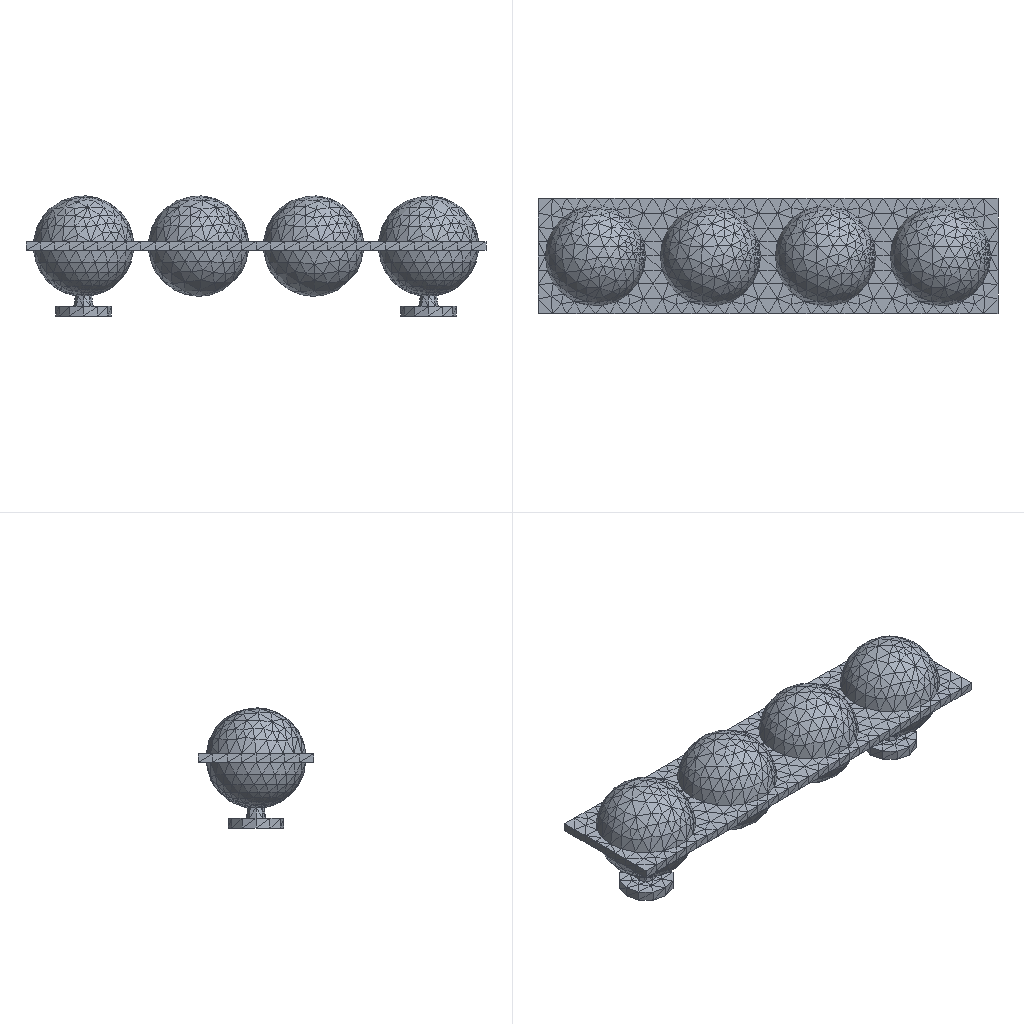Simulation study | abaqus
Set-up summary:
category,name,step,type,value,unit,region
solver,abaqus
solver,version,,,Abaqus/Standard 2020
units,not stated in the deck,,not stated
analysis,deck,,transient,transient
load_step,Step-1,Step-1,transient
load_step,Step-2,Step-2,transient
load_step,Step-3,Step-3,transient
load_step,Step-4,Step-4,transient
load_step,Step-5,Step-5,transient
load_step,Step-6,Step-6,transient
load_step,Step-7,Step-7,transient
load_step,Step-8,Step-8,transient
load_step,requested,,,8
mesh,nodes,,,2127
mesh,elements,,,6350
element_type,C3D4H,,solid,6350
load,load commands in deck,,count,10
bc,support commands in deck,,count,2
material,MATERIAL-1,,in results
check,setup vs results,,match,"per instance, exact: element labels, types and connectivity; labels of the nodes the elements use; coordinates of those nodes at SINGLE_PRECISION in 1 of 1 instance(s)"
Abaqus input file, long lists of numbers shortened:
*Heading
** Job name: Job-2 Model name: Model-1-Copy
** Generated by: Abaqus/CAE 2020
*Preprint, echo=NO, model=NO, history=NO, contact=NO
**
** PARTS
**
*Part, name=Part-4
*Node
      1,   116.804,           0.,  -34.854
      2,   123.196,           0.,  -34.854
** (2125 more lines like these left out)
*Element, type=C3D4H
   1, 2079, 2080,   17,   27
   2,  169, 2081, 1075, 1018
** (6348 more lines like these left out)
*Nset, nset=Set-4, generate
    1,  2127,     1
*Elset, elset=Set-4, generate
    1,  6350,     1
** Section: Section-1
*Solid Section, elset=Set-4, material=Material-1
,
*End Part
**
**
** ASSEMBLY
**
*Assembly, name=Assembly
**
*Instance, name=Part-4-1, part=Part-4
*End Instance
**
*Nset, nset=Set-1, instance=Part-4-1
  63,  64,  65,  66, 519, 520, 521, 522, 523, 524, 525, 526, 527, 528, 529, 530
 531, 532, 533, 534
*Elset, elset=Set-1, instance=Part-4-1
 3357, 3370, 3373, 3374, 3381, 3384, 3395, 3401, 3404, 3412, 3414, 3423, 3424, 3425, 3428, 3432
 3440, 3445, 3450, 3451
*Nset, nset=Set-2, instance=Part-4-1
   7,   8,   9,  10,  99, 100, 101, 102, 103, 104, 105, 106, 107, 108, 109, 110
 111, 112, 113, 114
*Elset, elset=Set-2, instance=Part-4-1
 2982, 2992, 2993, 3009, 3025, 3029, 3032, 3041, 3056, 3057, 3066, 3069, 3079, 3084, 3093, 3102
 3117, 3125, 3131, 3157
*Nset, nset=Set-3, instance=Part-4-1
  63,  64,  65,  66, 519, 520, 521, 522, 523, 524, 525, 526, 527, 528, 529, 530
 531, 532, 533, 534
*Elset, elset=Set-3, instance=Part-4-1
 3357, 3370, 3373, 3374, 3381, 3384, 3395, 3401, 3404, 3412, 3414, 3423, 3424, 3425, 3428, 3432
 3440, 3445, 3450, 3451
*Nset, nset=Set-4, instance=Part-4-1
   7,   8,   9,  10,  99, 100, 101, 102, 103, 104, 105, 106, 107, 108, 109, 110
 111, 112, 113, 114
*Elset, elset=Set-4, instance=Part-4-1
 2982, 2992, 2993, 3009, 3025, 3029, 3032, 3041, 3056, 3057, 3066, 3069, 3079, 3084, 3093, 3102
 3117, 3125, 3131, 3157
*Nset, nset=Set-5, instance=Part-4-1
  63,  64,  65,  66, 519, 520, 521, 522, 523, 524, 525, 526, 527, 528, 529, 530
 531, 532, 533, 534
*Elset, elset=Set-5, instance=Part-4-1
 3357, 3370, 3373, 3374, 3381, 3384, 3395, 3401, 3404, 3412, 3414, 3423, 3424, 3425, 3428, 3432
 3440, 3445, 3450, 3451
*Nset, nset=Set-6, instance=Part-4-1
   7,   8,   9,  10,  99, 100, 101, 102, 103, 104, 105, 106, 107, 108, 109, 110
 111, 112, 113, 114
*Elset, elset=Set-6, instance=Part-4-1
 2982, 2992, 2993, 3009, 3025, 3029, 3032, 3041, 3056, 3057, 3066, 3069, 3079, 3084, 3093, 3102
 3117, 3125, 3131, 3157
*Elset, elset=_Surf-1_S3, internal, instance=Part-4-1
   38,   82,   83,   98,  101,  102,  103,  178,  233,  238,  269,  271,  272, 1477, 1518, 1523
 1548, 1561, 1564, 1630, 1633, 1669, 1682, 1708, 1709, 1766, 1768, 1770, 1784, 1787, 1799, 1802
** (22 more lines like these left out)
*Elset, elset=_Surf-1_S4, internal, instance=Part-4-1
   39,   41,  630, 1513, 1600, 1821, 1840, 1843, 1905, 3464, 5248, 5324, 5368, 5438, 5474, 5518
 5533, 5703, 5804, 5953, 5978
*Elset, elset=_Surf-1_S1, internal, instance=Part-4-1
  236,  276, 1549, 1631, 1634, 1700, 2060, 2424, 3561, 5379, 5427, 5439, 5487, 5599, 5615, 5645
 5658, 5682, 5917, 5991
*Elset, elset=_Surf-1_S2, internal, instance=Part-4-1
  828, 1581, 1800, 1901, 1921, 1998, 2020, 2058, 2784, 5366, 5468, 5511, 5515, 5526, 5538, 5585
 5602, 5663, 5671, 5719, 5744, 5947, 5980, 6014
*Surface, type=ELEMENT, name=Surf-1
_Surf-1_S3, S3
_Surf-1_S4, S4
_Surf-1_S2, S2
_Surf-1_S1, S1
*Elset, elset=_Surf-2_S4, internal, instance=Part-4-1
   55,   57,   66, 2162, 2179, 2191, 2194, 2238, 2249, 2394, 2414, 2586, 2627, 2734, 2843, 3613
 3855, 3928, 3953, 3965, 3977, 4341, 4403, 4483
*Elset, elset=_Surf-2_S2, internal, instance=Part-4-1
   67, 1976, 2148, 2149, 2306, 2392, 2616, 2723, 2750, 2950, 2980, 3040, 3042, 3095, 3105, 3203
 3615, 3616, 3621, 3624, 3790, 3799, 3823, 3827, 3836, 3843, 3860, 3882, 3892, 3893, 3907, 3911
** (1 more lines like these left out)
*Elset, elset=_Surf-2_S3, internal, instance=Part-4-1
  148,  158,  248,  251,  252,  253,  255,  259,  262,  264,  266,  267,  268,  701, 1087, 2150
 2201, 2310, 2395, 2405, 2409, 2434, 2457, 2461, 2466, 2467, 2469, 2474, 2477, 2480, 2487, 2488
** (29 more lines like these left out)
*Elset, elset=_Surf-2_S1, internal, instance=Part-4-1
  149,  188,  256, 2313, 2339, 2730, 2775, 3481, 3612, 3883, 4087
*Surface, type=ELEMENT, name=Surf-2
_Surf-2_S4, S4
_Surf-2_S2, S2
_Surf-2_S3, S3
_Surf-2_S1, S1
*Elset, elset=_Surf-3_S3, internal, instance=Part-4-1
   26,   48,  141,  142,  171,  172,  173,  196,  197,  240,  242,  244,  245,  803,  804,  946
  947,  978, 1020, 1024, 1045, 1072, 1076, 1078, 1080, 1086, 1094, 1101, 1119, 1134, 1137, 1139
** (22 more lines like these left out)
*Elset, elset=_Surf-3_S4, internal, instance=Part-4-1
  131,  205,  642,  873,  884,  896,  921,  924,  977, 1002, 1035, 1093, 1100, 1175, 1227, 1268
 1425, 4412, 4523, 4536, 4668, 4775, 4796, 4799, 4893, 5139, 5172, 5711, 5914
*Elset, elset=_Surf-3_S2, internal, instance=Part-4-1
  169,  241, 1029, 1254, 1327, 4774, 4810, 4889, 5092, 5825, 5873, 6028, 6055
*Elset, elset=_Surf-3_S1, internal, instance=Part-4-1
  198,  201,  857,  950,  952, 1042, 1168, 1267, 1418, 4520, 4574, 4813, 4891, 4969, 5012, 5089
 5816, 5862
*Surface, type=ELEMENT, name=Surf-3
_Surf-3_S3, S3
_Surf-3_S4, S4
_Surf-3_S2, S2
_Surf-3_S1, S1
*Elset, elset=_Surf-4_S3, internal, instance=Part-4-1
   61,  109,  117,  225,  229,  232,  305,  319,  321,  351,  359,  384,  412,  413,  423,  424
  427,  436,  437,  444,  449,  484,  486,  495,  503,  510,  516,  518,  520,  555,  556,  560
** (30 more lines like these left out)
*Elset, elset=_Surf-4_S4, internal, instance=Part-4-1
    2,   28,  224,  297,  346,  396,  451,  540,  542,  563,  571,  778,  793, 1792, 2125, 2305
 2459, 2646, 3160, 4894, 5064, 5102, 5751, 5838, 6214, 6346
*Elset, elset=_Surf-4_S1, internal, instance=Part-4-1
   10,   59,  122,  442,  652,  659,  783,  840, 1036, 2777, 2986, 3729, 4063, 4506, 4542, 4947
 5945,
*Elset, elset=_Surf-4_S2, internal, instance=Part-4-1
  231,  781,  994, 1125, 1514, 1865, 2039, 2766, 2817, 2957, 3072, 3606, 3723, 4623, 4741, 4762
 4817, 4819, 4897, 5008, 5046, 5443, 6135, 6156, 6316
*Surface, type=ELEMENT, name=Surf-4
_Surf-4_S3, S3
_Surf-4_S4, S4
_Surf-4_S2, S2
_Surf-4_S1, S1
*Elset, elset=_Surf-6_S2, internal, instance=Part-4-1
  275, 1467, 1472, 1476, 1482, 1487, 1494, 1498, 1501, 1512, 1521, 1551, 1558, 1563, 1565, 1572
 1573, 1578, 1584, 1589, 1594, 1596, 1598, 1607, 1614, 1617, 1619, 1624, 1641, 1644, 1650, 1654
** (5 more lines like these left out)
*Elset, elset=_Surf-6_S4, internal, instance=Part-4-1
 1480, 1503, 1541, 1554, 1579, 1583, 1586, 1591, 1597, 1602, 1615, 1626, 1628, 1639, 1640, 1655
 1676, 1678, 1686, 1695, 1731, 1744, 1745, 1778, 1783, 1793, 1794, 1811, 1817, 1879, 1882, 1902
** (2 more lines like these left out)
*Elset, elset=_Surf-6_S1, internal, instance=Part-4-1
 1485, 1488, 1496, 1497, 1502, 1507, 1517, 1528, 1535, 1555, 1566, 1570, 1592, 1601, 1603, 1606
 1608, 1632, 1647, 1649, 1668, 1673, 1674, 1689, 1693, 1702, 1710, 1714, 1725, 1740, 1743, 1754
** (3 more lines like these left out)
*Elset, elset=_Surf-6_S3, internal, instance=Part-4-1
 1486, 1505, 1567, 1694, 1805, 1810, 1812, 1886, 1970, 1983, 2031, 2061, 5649
*Surface, type=ELEMENT, name=Surf-6
_Surf-6_S2, S2
_Surf-6_S4, S4
_Surf-6_S1, S1
_Surf-6_S3, S3
*Elset, elset=_Surf-9_S2, internal, instance=Part-4-1
  801,  806,  810,  819,  827,  831,  836,  849,  861,  862,  870,  871,  885,  889,  890,  899
  900,  908,  913,  915,  916,  919,  936,  937,  938,  939,  943,  945,  961,  968,  970,  972
** (5 more lines like these left out)
*Elset, elset=_Surf-9_S1, internal, instance=Part-4-1
  805,  807,  813,  814,  818,  829,  830,  833,  837,  847,  853,  859,  864,  866,  875,  886
  897,  902,  905,  931,  941,  956,  958,  959,  974,  984,  989, 1000, 1017, 1034, 1039, 1063
** (3 more lines like these left out)
*Elset, elset=_Surf-9_S4, internal, instance=Part-4-1
  809,  821,  839,  851,  868,  879,  909,  914,  935,  949,  951,  955,  965,  981, 1026, 1031
 1065, 1074, 1098, 1109, 1121, 1126, 1142, 1146, 1152, 1164, 1177, 1180, 1224, 1234, 1253, 1257
** (2 more lines like these left out)
*Elset, elset=_Surf-9_S3, internal, instance=Part-4-1
  838,  841,  966, 1122, 1155, 1205, 1311, 1316, 1344, 1458, 2728, 3870, 4904, 5887, 6086, 6122
*Surface, type=ELEMENT, name=Surf-9
_Surf-9_S2, S2
_Surf-9_S1, S1
_Surf-9_S4, S4
_Surf-9_S3, S3
*Elset, elset=_Surf-10_S2, internal, instance=Part-4-1
   78,  204,  309,  312,  313,  318,  320,  330,  339,  340,  347,  354,  355,  357,  360,  365
  372,  374,  382,  389,  398,  400,  406,  410,  414,  416,  422,  430,  443,  445,  460,  472
** (6 more lines like these left out)
*Elset, elset=_Surf-10_S4, internal, instance=Part-4-1
  307,  310,  325,  349,  353,  358,  361,  379,  405,  419,  426,  450,  464,  505,  521,  531
  535,  602,  614,  641,  653,  657,  679,  696,  734,  763,  768,  811,  933, 1033, 1240, 1575
** (2 more lines like these left out)
*Elset, elset=_Surf-10_S1, internal, instance=Part-4-1
  308,  331,  336,  367,  385,  397,  418,  428,  440,  448,  461,  478,  479,  501,  513,  517
  532,  546,  566,  569,  585,  590,  603,  609,  624,  631,  637,  656,  677,  685,  694,  699
** (3 more lines like these left out)
*Elset, elset=_Surf-10_S3, internal, instance=Part-4-1
  329,  363,  364,  465,  474,  538,  686,  698,  907, 1337, 2126, 2135, 5563, 6035, 6327
*Surface, type=ELEMENT, name=Surf-10
_Surf-10_S2, S2
_Surf-10_S4, S4
_Surf-10_S1, S1
_Surf-10_S3, S3
*Elset, elset=_Surf-12_S2, internal, instance=Part-4-1
   63,  749, 2142, 2151, 2157, 2159, 2161, 2182, 2193, 2211, 2214, 2223, 2230, 2234, 2237, 2246
 2247, 2251, 2252, 2261, 2269, 2276, 2284, 2304, 2322, 2326, 2330, 2331, 2341, 2343, 2346, 2350
** (5 more lines like these left out)
*Elset, elset=_Surf-12_S3, internal, instance=Part-4-1
  182, 2156, 2290, 2319, 2352, 2358, 2360, 2425, 2541, 2642, 2762, 2874, 3073, 3794
*Elset, elset=_Surf-12_S4, internal, instance=Part-4-1
 2144, 2165, 2204, 2207, 2228, 2235, 2242, 2253, 2258, 2273, 2280, 2281, 2287, 2295, 2308, 2309
 2311, 2314, 2316, 2348, 2408, 2411, 2444, 2482, 2498, 2520, 2529, 2557, 2609, 2640, 2655, 2715
** (2 more lines like these left out)
*Elset, elset=_Surf-12_S1, internal, instance=Part-4-1
 2147, 2160, 2167, 2168, 2187, 2188, 2189, 2195, 2209, 2212, 2215, 2233, 2259, 2267, 2271, 2288
 2289, 2298, 2321, 2337, 2340, 2355, 2368, 2383, 2415, 2418, 2440, 2450, 2517, 2532, 2537, 2558
** (3 more lines like these left out)
*Surface, type=ELEMENT, name=Surf-12
_Surf-12_S2, S2
_Surf-12_S3, S3
_Surf-12_S4, S4
_Surf-12_S1, S1
*Elset, elset=_Surf-13_S2, internal, instance=Part-4-1
  275, 1467, 1472, 1476, 1482, 1487, 1494, 1498, 1501, 1512, 1521, 1551, 1558, 1563, 1565, 1572
 1573, 1578, 1584, 1589, 1594, 1596, 1598, 1607, 1614, 1617, 1619, 1624, 1641, 1644, 1650, 1654
** (5 more lines like these left out)
*Elset, elset=_Surf-13_S4, internal, instance=Part-4-1
 1480, 1503, 1541, 1554, 1579, 1583, 1586, 1591, 1597, 1602, 1615, 1626, 1628, 1639, 1640, 1655
 1676, 1678, 1686, 1695, 1731, 1744, 1745, 1778, 1783, 1793, 1794, 1811, 1817, 1879, 1882, 1902
** (2 more lines like these left out)
*Elset, elset=_Surf-13_S1, internal, instance=Part-4-1
 1485, 1488, 1496, 1497, 1502, 1507, 1517, 1528, 1535, 1555, 1566, 1570, 1592, 1601, 1603, 1606
 1608, 1632, 1647, 1649, 1668, 1673, 1674, 1689, 1693, 1702, 1710, 1714, 1725, 1740, 1743, 1754
** (3 more lines like these left out)
*Elset, elset=_Surf-13_S3, internal, instance=Part-4-1
 1486, 1505, 1567, 1694, 1805, 1810, 1812, 1886, 1970, 1983, 2031, 2061, 5649
*Surface, type=ELEMENT, name=Surf-13
_Surf-13_S2, S2
_Surf-13_S4, S4
_Surf-13_S1, S1
_Surf-13_S3, S3
*Elset, elset=_Surf-14_S2, internal, instance=Part-4-1
   63,  749, 2142, 2151, 2157, 2159, 2161, 2182, 2193, 2211, 2214, 2223, 2230, 2234, 2237, 2246
 2247, 2251, 2252, 2261, 2269, 2276, 2284, 2304, 2322, 2326, 2330, 2331, 2341, 2343, 2346, 2350
** (5 more lines like these left out)
*Elset, elset=_Surf-14_S3, internal, instance=Part-4-1
  182, 2156, 2290, 2319, 2352, 2358, 2360, 2425, 2541, 2642, 2762, 2874, 3073, 3794
*Elset, elset=_Surf-14_S4, internal, instance=Part-4-1
 2144, 2165, 2204, 2207, 2228, 2235, 2242, 2253, 2258, 2273, 2280, 2281, 2287, 2295, 2308, 2309
 2311, 2314, 2316, 2348, 2408, 2411, 2444, 2482, 2498, 2520, 2529, 2557, 2609, 2640, 2655, 2715
** (2 more lines like these left out)
*Elset, elset=_Surf-14_S1, internal, instance=Part-4-1
 2147, 2160, 2167, 2168, 2187, 2188, 2189, 2195, 2209, 2212, 2215, 2233, 2259, 2267, 2271, 2288
 2289, 2298, 2321, 2337, 2340, 2355, 2368, 2383, 2415, 2418, 2440, 2450, 2517, 2532, 2537, 2558
** (3 more lines like these left out)
*Surface, type=ELEMENT, name=Surf-14
_Surf-14_S2, S2
_Surf-14_S3, S3
_Surf-14_S4, S4
_Surf-14_S1, S1
*Elset, elset=_Surf-15_S2, internal, instance=Part-4-1
  801,  806,  810,  819,  827,  831,  836,  849,  861,  862,  870,  871,  885,  889,  890,  899
  900,  908,  913,  915,  916,  919,  936,  937,  938,  939,  943,  945,  961,  968,  970,  972
** (5 more lines like these left out)
*Elset, elset=_Surf-15_S1, internal, instance=Part-4-1
  805,  807,  813,  814,  818,  829,  830,  833,  837,  847,  853,  859,  864,  866,  875,  886
  897,  902,  905,  931,  941,  956,  958,  959,  974,  984,  989, 1000, 1017, 1034, 1039, 1063
** (3 more lines like these left out)
*Elset, elset=_Surf-15_S4, internal, instance=Part-4-1
  809,  821,  839,  851,  868,  879,  909,  914,  935,  949,  951,  955,  965,  981, 1026, 1031
 1065, 1074, 1098, 1109, 1121, 1126, 1142, 1146, 1152, 1164, 1177, 1180, 1224, 1234, 1253, 1257
** (2 more lines like these left out)
*Elset, elset=_Surf-15_S3, internal, instance=Part-4-1
  838,  841,  966, 1122, 1155, 1205, 1311, 1316, 1344, 1458, 2728, 3870, 4904, 5887, 6086, 6122
*Surface, type=ELEMENT, name=Surf-15
_Surf-15_S2, S2
_Surf-15_S1, S1
_Surf-15_S4, S4
_Surf-15_S3, S3
*Elset, elset=_Surf-16_S2, internal, instance=Part-4-1
   78,  204,  309,  312,  313,  318,  320,  330,  339,  340,  347,  354,  355,  357,  360,  365
  372,  374,  382,  389,  398,  400,  406,  410,  414,  416,  422,  430,  443,  445,  460,  472
** (6 more lines like these left out)
*Elset, elset=_Surf-16_S4, internal, instance=Part-4-1
  307,  310,  325,  349,  353,  358,  361,  379,  405,  419,  426,  450,  464,  505,  521,  531
  535,  602,  614,  641,  653,  657,  679,  696,  734,  763,  768,  811,  933, 1033, 1240, 1575
** (2 more lines like these left out)
*Elset, elset=_Surf-16_S1, internal, instance=Part-4-1
  308,  331,  336,  367,  385,  397,  418,  428,  440,  448,  461,  478,  479,  501,  513,  517
  532,  546,  566,  569,  585,  590,  603,  609,  624,  631,  637,  656,  677,  685,  694,  699
** (3 more lines like these left out)
*Elset, elset=_Surf-16_S3, internal, instance=Part-4-1
  329,  363,  364,  465,  474,  538,  686,  698,  907, 1337, 2126, 2135, 5563, 6035, 6327
*Surface, type=ELEMENT, name=Surf-16
_Surf-16_S2, S2
_Surf-16_S4, S4
_Surf-16_S1, S1
_Surf-16_S3, S3
*Elset, elset=__Int-1_gcs0_1_S1, internal, instance=Part-4-1
   44, 2905
*Elset, elset=__Int-1_gcs0_1_S2, internal, instance=Part-4-1
 2803, 2837
*Elset, elset=__Int-1_gcs0_1_S3, internal, instance=Part-4-1
 2904, 2906, 2965, 3661
*Surface, type=ELEMENT, name=_Int-1_gcs0_1, internal
__Int-1_gcs0_1_S1, S1
__Int-1_gcs0_1_S2, S2
__Int-1_gcs0_1_S3, S3
*Elset, elset=__Int-1_gcs0_2_S3, internal, instance=Part-4-1
 2630, 3014, 3032, 3041, 3057, 3061, 3116, 3117
*Surface, type=ELEMENT, name=_Int-1_gcs0_2, internal
__Int-1_gcs0_2_S3, S3
*Elset, elset=__Int-1_gcs0_3_S2, internal, instance=Part-4-1
 2946, 3141, 3446
*Elset, elset=__Int-1_gcs0_3_S4, internal, instance=Part-4-1
 2969, 3435, 3436, 3459
*Elset, elset=__Int-1_gcs0_3_S3, internal, instance=Part-4-1
 3133, 3156
*Elset, elset=__Int-1_gcs0_3_S1, internal, instance=Part-4-1
 3150, 3439, 3442
*Surface, type=ELEMENT, name=_Int-1_gcs0_3, internal
__Int-1_gcs0_3_S2, S2
__Int-1_gcs0_3_S4, S4
__Int-1_gcs0_3_S3, S3
__Int-1_gcs0_3_S1, S1
*Elset, elset=__Int-1_gcs0_4_S1, internal, instance=Part-4-1
 2963, 2997, 3683, 4183
*Elset, elset=__Int-1_gcs0_4_S3, internal, instance=Part-4-1
 2971,
*Elset, elset=__Int-1_gcs0_4_S4, internal, instance=Part-4-1
 3694, 4232
*Elset, elset=__Int-1_gcs0_4_S2, internal, instance=Part-4-1
 3735,
*Surface, type=ELEMENT, name=_Int-1_gcs0_4, internal
__Int-1_gcs0_4_S1, S1
__Int-1_gcs0_4_S3, S3
__Int-1_gcs0_4_S4, S4
__Int-1_gcs0_4_S2, S2
*Elset, elset=__Int-1_gcs0_5_S3, internal, instance=Part-4-1
  114, 3300, 3664
*Elset, elset=__Int-1_gcs0_5_S1, internal, instance=Part-4-1
 2696, 3144
*Elset, elset=__Int-1_gcs0_5_S2, internal, instance=Part-4-1
 3152, 3286
*Elset, elset=__Int-1_gcs0_5_S4, internal, instance=Part-4-1
 3155,
*Surface, type=ELEMENT, name=_Int-1_gcs0_5, internal
__Int-1_gcs0_5_S3, S3
__Int-1_gcs0_5_S1, S1
__Int-1_gcs0_5_S2, S2
__Int-1_gcs0_5_S4, S4
*Elset, elset=__Int-1_gcs0_6_S2, internal, instance=Part-4-1
 3391, 3407, 3414, 3422, 3425
*Elset, elset=__Int-1_gcs0_6_S4, internal, instance=Part-4-1
 3438,
*Elset, elset=__Int-1_gcs0_6_S1, internal, instance=Part-4-1
 3445, 3450
*Surface, type=ELEMENT, name=_Int-1_gcs0_6, internal
__Int-1_gcs0_6_S2, S2
__Int-1_gcs0_6_S4, S4
__Int-1_gcs0_6_S1, S1
*Elset, elset=__Int-1_gcs0_7_S3, internal, instance=Part-4-1
 2682, 3457, 3463, 3475, 3500, 3504, 3506, 3508, 3510, 3551, 4077
*Elset, elset=__Int-1_gcs0_7_S1, internal, instance=Part-4-1
 3505,
*Surface, type=ELEMENT, name=_Int-1_gcs0_7, internal
__Int-1_gcs0_7_S3, S3
__Int-1_gcs0_7_S1, S1
*Elset, elset=__Int-1_gcs0_8_S3, internal, instance=Part-4-1
 3579, 3581, 3630, 3702, 3825, 4152
*Elset, elset=__Int-1_gcs0_8_S1, internal, instance=Part-4-1
 3888, 4571
*Surface, type=ELEMENT, name=_Int-1_gcs0_8, internal
__Int-1_gcs0_8_S3, S3
__Int-1_gcs0_8_S1, S1
*Elset, elset=__Int-1_gcs0_9_S3, internal, instance=Part-4-1
   53, 2755, 3158, 3172, 3843, 3851
*Elset, elset=__Int-1_gcs0_9_S4, internal, instance=Part-4-1
 3167,
*Elset, elset=__Int-1_gcs0_9_S1, internal, instance=Part-4-1
 3471,
*Surface, type=ELEMENT, name=_Int-1_gcs0_9, internal
__Int-1_gcs0_9_S3, S3
__Int-1_gcs0_9_S4, S4
__Int-1_gcs0_9_S1, S1
*Elset, elset=__Int-1_gcs0_10_S1, internal, instance=Part-4-1
 128,
*Elset, elset=__Int-1_gcs0_10_S3, internal, instance=Part-4-1
 2563, 3225, 3516, 3524, 4600
*Elset, elset=__Int-1_gcs0_10_S2, internal, instance=Part-4-1
 3261,
*Elset, elset=__Int-1_gcs0_10_S4, internal, instance=Part-4-1
 4610,
*Surface, type=ELEMENT, name=_Int-1_gcs0_10, internal
__Int-1_gcs0_10_S1, S1
__Int-1_gcs0_10_S3, S3
__Int-1_gcs0_10_S2, S2
__Int-1_gcs0_10_S4, S4
*Elset, elset=__Int-1_gcs0_11_S3, internal, instance=Part-4-1
   43, 2437, 3553, 3560, 5394, 5421
*Elset, elset=__Int-1_gcs0_11_S2, internal, instance=Part-4-1
 239,
*Elset, elset=__Int-1_gcs0_11_S1, internal, instance=Part-4-1
 3464,
*Surface, type=ELEMENT, name=_Int-1_gcs0_11, internal
__Int-1_gcs0_11_S3, S3
__Int-1_gcs0_11_S2, S2
__Int-1_gcs0_11_S1, S1
*Elset, elset=__Int-1_gcs0_12_S2, internal, instance=Part-4-1
 47,
*Elset, elset=__Int-1_gcs0_12_S1, internal, instance=Part-4-1
 297,
*Elset, elset=__Int-1_gcs0_12_S3, internal, instance=Part-4-1
  301, 1125, 3350, 3614, 3619, 3634
*Surface, type=ELEMENT, name=_Int-1_gcs0_12, internal
__Int-1_gcs0_12_S2, S2
__Int-1_gcs0_12_S1, S1
__Int-1_gcs0_12_S3, S3
*Elset, elset=__Int-1_gcs0_13_S3, internal, instance=Part-4-1
  351,  384,  444,  757,  762,  764,  767,  769,  770,  771,  780,  782,  791,  795,  797,  798
  799,  967, 1447, 2385, 2470, 2645, 2677, 2788, 2799, 2801, 2821, 2824, 2851, 2925, 3134, 3137
** (16 more lines like these left out)
*Elset, elset=__Int-1_gcs0_13_S4, internal, instance=Part-4-1
  396,  540,  542,  778,  793, 4894, 5064
*Elset, elset=__Int-1_gcs0_13_S1, internal, instance=Part-4-1
  659,  783, 4506, 4542
*Elset, elset=__Int-1_gcs0_13_S2, internal, instance=Part-4-1
  781, 2817, 2957, 4623, 4762, 4817, 4819, 4897, 5046, 6156
*Surface, type=ELEMENT, name=_Int-1_gcs0_13, internal
__Int-1_gcs0_13_S3, S3
__Int-1_gcs0_13_S4, S4
__Int-1_gcs0_13_S2, S2
__Int-1_gcs0_13_S1, S1
*Elset, elset=__Int-1_gcs0_14_S4, internal, instance=Part-4-1
 2179, 2191, 2194, 2238, 2249, 2414, 3613, 3855, 3928, 3953, 4403
*Elset, elset=__Int-1_gcs0_14_S2, internal, instance=Part-4-1
 2392, 2616, 2950, 3095, 3105, 3615, 3616, 3621, 3624, 3790, 3799, 3893, 3911, 3923, 4003
*Elset, elset=__Int-1_gcs0_14_S3, internal, instance=Part-4-1
 2395, 2405, 2434, 2474, 2487, 2540, 2613, 2674, 2683, 2684, 2685, 2686, 2695, 2698, 2699, 2702
 2707, 2709, 2719, 2731, 2733, 2840, 2852, 2890, 2892, 2915, 2927, 2931, 2936, 2952, 3001, 3008
** (15 more lines like these left out)
*Elset, elset=__Int-1_gcs0_14_S1, internal, instance=Part-4-1
 2730, 3612
*Surface, type=ELEMENT, name=_Int-1_gcs0_14, internal
__Int-1_gcs0_14_S4, S4
__Int-1_gcs0_14_S2, S2
__Int-1_gcs0_14_S3, S3
__Int-1_gcs0_14_S1, S1
*Elset, elset=__Int-1_gcs0_15_S4, internal, instance=Part-4-1
   55,   57,   66, 2162, 2394, 2586, 2627, 2734, 2843, 3965, 3977, 4341, 4483
*Elset, elset=__Int-1_gcs0_15_S2, internal, instance=Part-4-1
   67, 1976, 2148, 2149, 2306, 2723, 2750, 2980, 3040, 3042, 3203, 3823, 3827, 3836, 3843, 3860
 3882, 3892, 3907, 3912, 4201, 4211, 4221, 4457, 4485
*Elset, elset=__Int-1_gcs0_15_S3, internal, instance=Part-4-1
  148,  158,  248,  251,  252,  253,  255,  259,  262,  264,  266,  267,  268,  701, 1087, 2150
 2201, 2310, 2409, 2457, 2461, 2466, 2467, 2469, 2477, 2480, 2488, 2490, 2501, 2504, 2507, 2510
** (12 more lines like these left out)
*Elset, elset=__Int-1_gcs0_15_S1, internal, instance=Part-4-1
  149,  188,  256, 2313, 2339, 2775, 3481, 3883, 4087
*Surface, type=ELEMENT, name=_Int-1_gcs0_15, internal
__Int-1_gcs0_15_S4, S4
__Int-1_gcs0_15_S2, S2
__Int-1_gcs0_15_S3, S3
__Int-1_gcs0_15_S1, S1
*Elset, elset=__Int-1_gcs0_16_S3, internal, instance=Part-4-1
   26,   48,  141,  142,  171,  172,  173,  196,  197,  240,  242,  244,  245,  803,  804,  978
 1020, 1072, 1076, 1078, 1080, 1086, 1094, 1101, 1134, 1137, 1139, 1140, 1165, 1166, 1170, 1173
** (13 more lines like these left out)
*Elset, elset=__Int-1_gcs0_16_S4, internal, instance=Part-4-1
  131,  205,  642,  977, 1002, 1093, 1100, 1175, 1227, 1268, 4412, 4536, 4668, 4775, 4796, 4799
 4893, 5139, 5172
*Elset, elset=__Int-1_gcs0_16_S2, internal, instance=Part-4-1
  169,  241, 1254, 1327, 4774, 4810, 4889, 5092
*Elset, elset=__Int-1_gcs0_16_S1, internal, instance=Part-4-1
  198,  201,  857,  950,  952, 1168, 1267, 4813, 4891, 4969, 5012, 5089, 5816
*Surface, type=ELEMENT, name=_Int-1_gcs0_16, internal
__Int-1_gcs0_16_S3, S3
__Int-1_gcs0_16_S4, S4
__Int-1_gcs0_16_S2, S2
__Int-1_gcs0_16_S1, S1
*Elset, elset=__Int-1_gcs0_17_S3, internal, instance=Part-4-1
   38,   82,   83,   98,  101,  102,  103,  178,  233,  238,  269,  271,  272, 1477, 1630, 1633
 1669, 1682, 1708, 1766, 1768, 1770, 1799, 1802, 1824, 1876, 1877, 1885, 1892, 1894, 1895, 1896
** (13 more lines like these left out)
*Elset, elset=__Int-1_gcs0_17_S4, internal, instance=Part-4-1
   39,   41,  630, 1821, 1905, 3464, 5248, 5474, 5533, 5703, 5804, 5978
*Elset, elset=__Int-1_gcs0_17_S1, internal, instance=Part-4-1
  236,  276, 1631, 1634, 2060, 3561, 5379, 5427, 5439, 5599, 5615, 5658, 5682, 5991
*Elset, elset=__Int-1_gcs0_17_S2, internal, instance=Part-4-1
  828, 1800, 1901, 1998, 2058, 2784, 5468, 5515, 5585, 5602, 5671, 5719, 5744, 5947, 5980, 6014
*Surface, type=ELEMENT, name=_Int-1_gcs0_17, internal
__Int-1_gcs0_17_S3, S3
__Int-1_gcs0_17_S4, S4
__Int-1_gcs0_17_S2, S2
__Int-1_gcs0_17_S1, S1
*Elset, elset=__Int-1_gcs0_18_S4, internal, instance=Part-4-1
    2,   28,  224,  297,  346,  451,  563,  571, 1792, 2125, 2305, 2459, 2646, 3160, 5102, 5751
 5838, 6214, 6346
*Elset, elset=__Int-1_gcs0_18_S1, internal, instance=Part-4-1
   10,   59,  122,  442,  652,  840, 1036, 2777, 2986, 3729, 4063, 4947, 5945
*Elset, elset=__Int-1_gcs0_18_S3, internal, instance=Part-4-1
   61,  109,  117,  225,  229,  232,  305,  319,  321,  359,  412,  413,  423,  424,  427,  436
  437,  449,  484,  486,  495,  503,  510,  516,  518,  520,  555,  556,  560,  564,  565,  568
** (12 more lines like these left out)
*Elset, elset=__Int-1_gcs0_18_S2, internal, instance=Part-4-1
  231,  994, 1125, 1514, 1865, 2039, 2766, 3072, 3606, 3723, 4741, 5008, 5443, 6135, 6316
*Surface, type=ELEMENT, name=_Int-1_gcs0_18, internal
__Int-1_gcs0_18_S4, S4
__Int-1_gcs0_18_S1, S1
__Int-1_gcs0_18_S2, S2
__Int-1_gcs0_18_S3, S3
*Elset, elset=__Int-1_gcs0_25_S4, internal, instance=Part-4-1
  873,  884,  896,  921,  924, 1035, 1425, 4523, 5711, 5914
*Elset, elset=__Int-1_gcs0_25_S3, internal, instance=Part-4-1
  946,  947, 1024, 1045, 1119, 1324, 1335, 1340, 1342, 1358, 1360, 1367, 1371, 1373, 1387, 1411
 1428, 1433, 1439, 1445, 1446, 1452, 1454, 1459, 1460, 1461, 1462, 1463, 1465, 2464, 2550, 2672
** (8 more lines like these left out)
*Elset, elset=__Int-1_gcs0_25_S2, internal, instance=Part-4-1
 1029, 5825, 5873, 6028, 6055
*Elset, elset=__Int-1_gcs0_25_S1, internal, instance=Part-4-1
 1042, 1418, 4520, 4574, 5862
*Surface, type=ELEMENT, name=_Int-1_gcs0_25, internal
__Int-1_gcs0_25_S4, S4
__Int-1_gcs0_25_S3, S3
__Int-1_gcs0_25_S2, S2
__Int-1_gcs0_25_S1, S1
*Elset, elset=__Int-1_gcs0_26_S4, internal, instance=Part-4-1
 1513, 1600, 1840, 1843, 5324, 5368, 5438, 5518, 5953
*Elset, elset=__Int-1_gcs0_26_S3, internal, instance=Part-4-1
 1518, 1523, 1548, 1561, 1564, 1709, 1784, 1787, 1836, 1845, 1851, 1852, 1925, 1932, 1942, 1957
 1969, 1972, 1981, 1987, 1994, 1999, 2005, 2015, 2030, 2043, 2052, 2054, 2055, 2068, 2072, 2093
** (8 more lines like these left out)
*Elset, elset=__Int-1_gcs0_26_S1, internal, instance=Part-4-1
 1549, 1700, 2424, 5487, 5645, 5917
*Elset, elset=__Int-1_gcs0_26_S2, internal, instance=Part-4-1
 1581, 1921, 2020, 5366, 5511, 5526, 5538, 5663
*Surface, type=ELEMENT, name=_Int-1_gcs0_26, internal
__Int-1_gcs0_26_S4, S4
__Int-1_gcs0_26_S3, S3
__Int-1_gcs0_26_S2, S2
__Int-1_gcs0_26_S1, S1
*Elset, elset=__Int-1_gcs0_27_S4, internal, instance=Part-4-1
 492,
*Elset, elset=__Int-1_gcs0_27_S3, internal, instance=Part-4-1
 1310, 2600, 2790, 3632, 3638, 6177, 6229
*Surface, type=ELEMENT, name=_Int-1_gcs0_27, internal
__Int-1_gcs0_27_S4, S4
__Int-1_gcs0_27_S3, S3
*Elset, elset=__Int-1_gcs0_29_S4, internal, instance=Part-4-1
 179, 221
*Elset, elset=__Int-1_gcs0_29_S3, internal, instance=Part-4-1
 2432, 3586, 3587, 3594, 5436, 5572
*Surface, type=ELEMENT, name=_Int-1_gcs0_29, internal
__Int-1_gcs0_29_S4, S4
__Int-1_gcs0_29_S3, S3
*Elset, elset=__Int-1_gcs0_31_S4, internal, instance=Part-4-1
 22,
*Elset, elset=__Int-1_gcs0_31_S3, internal, instance=Part-4-1
 3220, 3239, 3539, 4613, 4621, 4639, 4758
*Surface, type=ELEMENT, name=_Int-1_gcs0_31, internal
__Int-1_gcs0_31_S4, S4
__Int-1_gcs0_31_S3, S3
*Elset, elset=__Int-1_gcs0_33_S3, internal, instance=Part-4-1
 2718, 3165, 3494, 3495, 4016, 4020
*Elset, elset=__Int-1_gcs0_33_S4, internal, instance=Part-4-1
 4001,
*Elset, elset=__Int-1_gcs0_33_S2, internal, instance=Part-4-1
 4004,
*Surface, type=ELEMENT, name=_Int-1_gcs0_33, internal
__Int-1_gcs0_33_S3, S3
__Int-1_gcs0_33_S4, S4
__Int-1_gcs0_33_S2, S2
*Elset, elset=__Int-1_gcs0_35_S3, internal, instance=Part-4-1
 2668, 3305, 3309, 3520, 3786, 3861
*Elset, elset=__Int-1_gcs0_35_S1, internal, instance=Part-4-1
 3149, 3313
*Surface, type=ELEMENT, name=_Int-1_gcs0_35, internal
__Int-1_gcs0_35_S3, S3
__Int-1_gcs0_35_S1, S1
*Elset, elset=__Int-1_gcs0_37_S3, internal, instance=Part-4-1
 3478, 3482, 3483, 3487, 3489, 3514, 3518, 3535, 3541, 4111, 4563, 6299
*Surface, type=ELEMENT, name=_Int-1_gcs0_37, internal
__Int-1_gcs0_37_S3, S3
*Elset, elset=__Int-1_gcs0_39_S4, internal, instance=Part-4-1
 3352, 3404
*Elset, elset=__Int-1_gcs0_39_S2, internal, instance=Part-4-1
 3374, 3381
*Elset, elset=__Int-1_gcs0_39_S1, internal, instance=Part-4-1
 3428, 3458, 3460, 3472
*Surface, type=ELEMENT, name=_Int-1_gcs0_39, internal
__Int-1_gcs0_39_S4, S4
__Int-1_gcs0_39_S2, S2
__Int-1_gcs0_39_S1, S1
*Elset, elset=__Int-1_gcs0_41_S2, internal, instance=Part-4-1
 2492, 3139, 3159, 3199
*Elset, elset=__Int-1_gcs0_41_S4, internal, instance=Part-4-1
 3121,
*Elset, elset=__Int-1_gcs0_41_S1, internal, instance=Part-4-1
 3135,
*Elset, elset=__Int-1_gcs0_41_S3, internal, instance=Part-4-1
 3190, 3289
*Surface, type=ELEMENT, name=_Int-1_gcs0_41, internal
__Int-1_gcs0_41_S2, S2
__Int-1_gcs0_41_S4, S4
__Int-1_gcs0_41_S1, S1
__Int-1_gcs0_41_S3, S3
*Elset, elset=__Int-1_gcs0_42_S3, internal, instance=Part-4-1
 3112, 3115, 3123, 3130, 3136, 3148, 3163, 3948
*Surface, type=ELEMENT, name=_Int-1_gcs0_42, internal
__Int-1_gcs0_42_S3, S3
*Elset, elset=__Int-1_gcs0_43_S3, internal, instance=Part-4-1
 1435, 2923, 3010, 4455
*Elset, elset=__Int-1_gcs0_43_S1, internal, instance=Part-4-1
 2849, 2900, 3417
*Elset, elset=__Int-1_gcs0_43_S2, internal, instance=Part-4-1
 3756,
*Surface, type=ELEMENT, name=_Int-1_gcs0_43, internal
__Int-1_gcs0_43_S3, S3
__Int-1_gcs0_43_S1, S1
__Int-1_gcs0_43_S2, S2
*Elset, elset=__Int-1_gcs0_45_S2, internal, instance=Part-4-1
 2813, 3053, 3060, 3103, 3402, 3416
*Elset, elset=__Int-1_gcs0_45_S3, internal, instance=Part-4-1
 2862, 3420
*Elset, elset=__Int-1_gcs0_45_S1, internal, instance=Part-4-1
 3128, 3399, 3713
*Elset, elset=__Int-1_gcs0_45_S4, internal, instance=Part-4-1
 3413,
*Surface, type=ELEMENT, name=_Int-1_gcs0_45, internal
__Int-1_gcs0_45_S2, S2
__Int-1_gcs0_45_S3, S3
__Int-1_gcs0_45_S4, S4
__Int-1_gcs0_45_S1, S1
*Elset, elset=__Int-1_gcs0_47_S3, internal, instance=Part-4-1
 2973, 3079, 3126, 3131, 3132, 3140
*Elset, elset=__Int-1_gcs0_47_S1, internal, instance=Part-4-1
 3025, 3066
*Surface, type=ELEMENT, name=_Int-1_gcs0_47, internal
__Int-1_gcs0_47_S3, S3
__Int-1_gcs0_47_S1, S1
*Elset, elset=__Int-1_gcs0_49_S3, internal, instance=Part-4-1
 1916, 2944, 3741
*Elset, elset=__Int-1_gcs0_49_S2, internal, instance=Part-4-1
 2832, 2875, 2935
*Elset, elset=__Int-1_gcs0_49_S4, internal, instance=Part-4-1
 2899, 2945
*Surface, type=ELEMENT, name=_Int-1_gcs0_49, internal
__Int-1_gcs0_49_S3, S3
__Int-1_gcs0_49_S2, S2
__Int-1_gcs0_49_S4, S4
*Elset, elset=__Int-1_gcs0_50_S3, internal, instance=Part-4-1
 2445, 2569, 2811, 2825, 2828, 2829, 3360, 3361
*Surface, type=ELEMENT, name=_Int-1_gcs0_50, internal
__Int-1_gcs0_50_S3, S3
*Elset, elset=__Int-1_gcs0_51_S2, internal, instance=Part-4-1
   78,  204,  309,  312,  313,  318,  320,  330,  339,  340,  347,  354,  355,  357,  360,  365
  372,  374,  382,  389,  398,  400,  406,  410,  414,  416,  422,  430,  443,  445,  460,  472
** (6 more lines like these left out)
*Elset, elset=__Int-1_gcs0_51_S4, internal, instance=Part-4-1
  307,  310,  325,  349,  353,  358,  361,  379,  405,  419,  426,  450,  464,  505,  521,  531
  535,  602,  614,  641,  653,  657,  679,  696,  734,  763,  768,  811,  933, 1033, 1240, 1575
** (2 more lines like these left out)
*Elset, elset=__Int-1_gcs0_51_S1, internal, instance=Part-4-1
  308,  331,  336,  367,  385,  397,  418,  428,  440,  448,  461,  478,  479,  501,  513,  517
  532,  546,  566,  569,  585,  590,  603,  609,  624,  631,  637,  656,  677,  685,  694,  699
** (3 more lines like these left out)
*Elset, elset=__Int-1_gcs0_51_S3, internal, instance=Part-4-1
  329,  363,  364,  465,  474,  538,  686,  698,  907, 1337, 2126, 2135, 5563, 6035, 6327
*Surface, type=ELEMENT, name=_Int-1_gcs0_51, internal
__Int-1_gcs0_51_S2, S2
__Int-1_gcs0_51_S4, S4
__Int-1_gcs0_51_S1, S1
__Int-1_gcs0_51_S3, S3
*Elset, elset=__Int-1_gcs0_52_S2, internal, instance=Part-4-1
  801,  806,  810,  819,  827,  831,  836,  849,  861,  862,  870,  871,  885,  889,  890,  899
  900,  908,  913,  915,  916,  919,  936,  937,  938,  939,  943,  945,  961,  968,  970,  972
** (5 more lines like these left out)
*Elset, elset=__Int-1_gcs0_52_S1, internal, instance=Part-4-1
  805,  807,  813,  814,  818,  829,  830,  833,  837,  847,  853,  859,  864,  866,  875,  886
  897,  902,  905,  931,  941,  956,  958,  959,  974,  984,  989, 1000, 1017, 1034, 1039, 1063
** (3 more lines like these left out)
*Elset, elset=__Int-1_gcs0_52_S4, internal, instance=Part-4-1
  809,  821,  839,  851,  868,  879,  909,  914,  935,  949,  951,  955,  965,  981, 1026, 1031
 1065, 1074, 1098, 1109, 1121, 1126, 1142, 1146, 1152, 1164, 1177, 1180, 1224, 1234, 1253, 1257
** (2 more lines like these left out)
*Elset, elset=__Int-1_gcs0_52_S3, internal, instance=Part-4-1
  838,  841,  966, 1122, 1155, 1205, 1311, 1316, 1344, 1458, 2728, 3870, 4904, 5887, 6086, 6122
*Surface, type=ELEMENT, name=_Int-1_gcs0_52, internal
__Int-1_gcs0_52_S2, S2
__Int-1_gcs0_52_S1, S1
__Int-1_gcs0_52_S4, S4
__Int-1_gcs0_52_S3, S3
*Elset, elset=__Int-1_gcs0_53_S2, internal, instance=Part-4-1
  275, 1467, 1472, 1476, 1482, 1487, 1494, 1498, 1501, 1512, 1521, 1551, 1558, 1563, 1565, 1572
 1573, 1578, 1584, 1589, 1594, 1596, 1598, 1607, 1614, 1617, 1619, 1624, 1641, 1644, 1650, 1654
** (5 more lines like these left out)
*Elset, elset=__Int-1_gcs0_53_S4, internal, instance=Part-4-1
 1480, 1503, 1541, 1554, 1579, 1583, 1586, 1591, 1597, 1602, 1615, 1626, 1628, 1639, 1640, 1655
 1676, 1678, 1686, 1695, 1731, 1744, 1745, 1778, 1783, 1793, 1794, 1811, 1817, 1879, 1882, 1902
** (2 more lines like these left out)
*Elset, elset=__Int-1_gcs0_53_S1, internal, instance=Part-4-1
 1485, 1488, 1496, 1497, 1502, 1507, 1517, 1528, 1535, 1555, 1566, 1570, 1592, 1601, 1603, 1606
 1608, 1632, 1647, 1649, 1668, 1673, 1674, 1689, 1693, 1702, 1710, 1714, 1725, 1740, 1743, 1754
** (3 more lines like these left out)
*Elset, elset=__Int-1_gcs0_53_S3, internal, instance=Part-4-1
 1486, 1505, 1567, 1694, 1805, 1810, 1812, 1886, 1970, 1983, 2031, 2061, 5649
*Surface, type=ELEMENT, name=_Int-1_gcs0_53, internal
__Int-1_gcs0_53_S2, S2
__Int-1_gcs0_53_S4, S4
__Int-1_gcs0_53_S1, S1
__Int-1_gcs0_53_S3, S3
*Elset, elset=__Int-1_gcs0_54_S2, internal, instance=Part-4-1
   63,  749, 2142, 2151, 2157, 2159, 2161, 2182, 2193, 2211, 2214, 2223, 2230, 2234, 2237, 2246
 2247, 2251, 2252, 2261, 2269, 2276, 2284, 2304, 2322, 2326, 2330, 2331, 2341, 2343, 2346, 2350
** (5 more lines like these left out)
*Elset, elset=__Int-1_gcs0_54_S3, internal, instance=Part-4-1
  182, 2156, 2290, 2319, 2352, 2358, 2360, 2425, 2541, 2642, 2762, 2874, 3073, 3794
*Elset, elset=__Int-1_gcs0_54_S4, internal, instance=Part-4-1
 2144, 2165, 2204, 2207, 2228, 2235, 2242, 2253, 2258, 2273, 2280, 2281, 2287, 2295, 2308, 2309
 2311, 2314, 2316, 2348, 2408, 2411, 2444, 2482, 2498, 2520, 2529, 2557, 2609, 2640, 2655, 2715
** (2 more lines like these left out)
*Elset, elset=__Int-1_gcs0_54_S1, internal, instance=Part-4-1
 2147, 2160, 2167, 2168, 2187, 2188, 2189, 2195, 2209, 2212, 2215, 2233, 2259, 2267, 2271, 2288
 2289, 2298, 2321, 2337, 2340, 2355, 2368, 2383, 2415, 2418, 2440, 2450, 2517, 2532, 2537, 2558
** (3 more lines like these left out)
*Surface, type=ELEMENT, name=_Int-1_gcs0_54, internal
__Int-1_gcs0_54_S2, S2
__Int-1_gcs0_54_S3, S3
__Int-1_gcs0_54_S4, S4
__Int-1_gcs0_54_S1, S1
*End Assembly
*Amplitude, name=Amp-1
             0.,              0.,              1.,              1.
**
** MATERIALS
**
*Material, name=Material-1
*Density
 1.1e-09,
*Hyperelastic, mooney-rivlin
 0.144, 0.036,    0.
**
** INTERACTION PROPERTIES
**
*Surface Interaction, name=IntProp-1
1.,
*Friction, slip tolerance=0.005
 0.1,
*Surface Behavior, pressure-overclosure=HARD
**
** INTERACTIONS
**
** Interaction: Int-1
*Contact
*Contact Inclusions, ALL EXTERIOR
*Contact Property Assignment
 ,  , IntProp-1
*Surface Property Assignment, property=GEOMETRIC CORRECTION
_Int-1_gcs0_1, Circumferential, 120., 0., 0.,  120., 0., -1.
_Int-1_gcs0_2, Circumferential, 120., 0., 0.,  120., 0., -1.
_Int-1_gcs0_3, Circumferential, 120., 0., 0.,  120., 0., -1.
_Int-1_gcs0_4, Circumferential, 120., 0., -34.544,  120., 0., -33.544
_Int-1_gcs0_5, Circumferential, -120., 0., 0.,  -120., 0., -1.
_Int-1_gcs0_6, Circumferential, -120., 0., 0.,  -120., 0., -1.
_Int-1_gcs0_7, Circumferential, -120., 0., 0.,  -120., 0., -1.
_Int-1_gcs0_8, Circumferential, -120., 0., -34.544,  -120., 0., -33.544
_Int-1_gcs0_9, Circumferential, -91., 0., 11.063,  -92., 0., 11.063
_Int-1_gcs0_10, Circumferential, -11., 0., 11.063,  -12., 0., 11.063
_Int-1_gcs0_11, Circumferential, 69., 0., 11.063,  68., 0., 11.063
_Int-1_gcs0_12, Circumferential, 149., 0., 11.063,  148., 0., 11.063
_Int-1_gcs0_13, Spherical, 120., 0., 0.
_Int-1_gcs0_14, Spherical, -120., 0., 0.
_Int-1_gcs0_15, Spherical, -120., 0., 0.
_Int-1_gcs0_16, Spherical, -40., 0., 0.
_Int-1_gcs0_17, Spherical, 40., 0., 0.
_Int-1_gcs0_18, Spherical, 120., 0., 0.
_Int-1_gcs0_25, Spherical, -40., 0., 0.
_Int-1_gcs0_26, Spherical, 40., 0., 0.
_Int-1_gcs0_27, Circumferential, 149., 0., 11.063,  148., 0., 11.063
_Int-1_gcs0_29, Circumferential, 69., 0., 11.063,  68., 0., 11.063
_Int-1_gcs0_31, Circumferential, -11., 0., 11.063,  -12., 0., 11.063
_Int-1_gcs0_33, Circumferential, -91., 0., 11.063,  -92., 0., 11.063
_Int-1_gcs0_35, Circumferential, -120., 0., -34.544,  -120., 0., -33.544
_Int-1_gcs0_37, Circumferential, -120., 0., 0.,  -120., 0., -1.
_Int-1_gcs0_39, Circumferential, -120., 0., 0.,  -120., 0., -1.
_Int-1_gcs0_41, Circumferential, -120., 0., 0.,  -120., 0., -1.
_Int-1_gcs0_42, Spherical, -120., 0., 0.
_Int-1_gcs0_43, Circumferential, 120., 0., -34.544,  120., 0., -33.544
_Int-1_gcs0_45, Circumferential, 120., 0., 0.,  120., 0., -1.
_Int-1_gcs0_47, Circumferential, 120., 0., 0.,  120., 0., -1.
_Int-1_gcs0_49, Circumferential, 120., 0., 0.,  120., 0., -1.
_Int-1_gcs0_50, Spherical, 120., 0., 0.
_Int-1_gcs0_51, Spherical, 120., 0.1288, 0.
_Int-1_gcs0_52, Spherical, -40., 0.1288, 0.
_Int-1_gcs0_53, Spherical, 40., 0.1288, 0.
_Int-1_gcs0_54, Spherical, -120., 0., -0.4
** ----------------------------------------------------------------
**
** STEP: Step-1
**
*Step, name=Step-1, nlgeom=YES, inc=1000
*Dynamic
0.001,1.,1e-05
**
** BOUNDARY CONDITIONS
**
** Name: BC-1 Type: 对称/反对称/完全固定
*Boundary
Set-5, ENCASTRE
**
** LOADS
**
** Name: Load-1   Type: Pressure
*Dsload, amplitude=Amp-1
Surf-13, P, 0.05
**
** OUTPUT REQUESTS
**
*Restart, write, frequency=0
**
** FIELD OUTPUT: F-Output-1
**
*Output, field, variable=PRESELECT, frequency=1
**
** HISTORY OUTPUT: H-Output-1
**
*Output, history, variable=PRESELECT, frequency=1
*End Step
** ----------------------------------------------------------------
**
** STEP: Step-2
**
*Step, name=Step-2, nlgeom=YES, inc=1000
*Dynamic
0.001,1.,1e-05
**
** LOADS
**
** Name: Load-2   Type: Pressure
*Dsload, amplitude=Amp-1
Surf-14, P, 0.05
**
** OUTPUT REQUESTS
**
*Restart, write, frequency=0
**
** FIELD OUTPUT: F-Output-1
**
*Output, field, variable=PRESELECT, frequency=1
**
** HISTORY OUTPUT: H-Output-1
**
*Output, history, variable=PRESELECT, frequency=1
*End Step
** ----------------------------------------------------------------
**
** STEP: Step-3
**
*Step, name=Step-3, nlgeom=YES, inc=1000
*Dynamic
0.001,1.,1e-05
**
** LOADS
**
** Name: Load-3   Type: Pressure
*Dsload, amplitude=Amp-1
Surf-15, P, 0.05
**
** OUTPUT REQUESTS
**
*Restart, write, frequency=0
**
** FIELD OUTPUT: F-Output-1
**
*Output, field, frequency=1
*Node Output
A, CF, RF, U, V
*Element Output, directions=YES
E, LE, MISES, PE, PEEQ, PEMAG, S
*Contact Output
CDISP, CSTRESS
**
** HISTORY OUTPUT: H-Output-1
**
*Output, history, variable=PRESELECT, frequency=1
*End Step
** ----------------------------------------------------------------
**
** STEP: Step-4
**
*Step, name=Step-4, nlgeom=YES, inc=1000
*Dynamic
0.001,1.,1e-05
**
** LOADS
**
** Name: Load-4   Type: Pressure
*Dsload, amplitude=Amp-1
Surf-16, P, 0.05
**
** OUTPUT REQUESTS
**
*Restart, write, frequency=0
**
** FIELD OUTPUT: F-Output-1
**
*Output, field, frequency=1
*Node Output
A, CF, RF, U, V
*Element Output, directions=YES
E, LE, MISES, PE, PEEQ, PEMAG, S
*Contact Output
CDISP, CSTRESS
**
** HISTORY OUTPUT: H-Output-1
**
*Output, history, variable=PRESELECT, frequency=1
*End Step
** ----------------------------------------------------------------
**
** STEP: Step-5
**
*Step, name=Step-5, nlgeom=YES, inc=1000
*Dynamic
0.001,1.,1e-05
**
** BOUNDARY CONDITIONS
**
** Name: BC-1 Type: 对称/反对称/完全固定
*Boundary, op=NEW
** Name: BC-2 Type: 对称/反对称/完全固定
*Boundary, op=NEW
Set-6, ENCASTRE
**
** LOADS
**
** Name: Load-1   Type: Pressure
*Dsload, op=NEW, amplitude=Amp-1
Surf-13, P, 0.05
** Name: Load-2   Type: Pressure
*Dsload, op=NEW
** Name: Load-3   Type: Pressure
*Dsload, op=NEW, amplitude=Amp-1
Surf-15, P, 0.05
** Name: Load-4   Type: Pressure
*Dsload, op=NEW, amplitude=Amp-1
Surf-16, P, 0.05
**
** OUTPUT REQUESTS
**
*Restart, write, frequency=0
**
** FIELD OUTPUT: F-Output-1
**
*Output, field, frequency=1
*Node Output
A, CF, RF, U, V
*Element Output, directions=YES
E, LE, MISES, PE, PEEQ, PEMAG, S
*Contact Output
CDISP, CSTRESS
**
** HISTORY OUTPUT: H-Output-1
**
*Output, history, variable=PRESELECT, frequency=1
*End Step
** ----------------------------------------------------------------
**
** STEP: Step-6
**
*Step, name=Step-6, nlgeom=YES, inc=1000
*Dynamic
0.001,1.,1e-05
**
** LOADS
**
** Name: Load-1   Type: Pressure
*Dsload, op=NEW
** Name: Load-3   Type: Pressure
*Dsload, op=NEW, amplitude=Amp-1
Surf-15, P, 0.05
** Name: Load-4   Type: Pressure
*Dsload, op=NEW, amplitude=Amp-1
Surf-16, P, 0.05
**
** OUTPUT REQUESTS
**
*Restart, write, frequency=0
**
** FIELD OUTPUT: F-Output-1
**
*Output, field, frequency=1
*Node Output
A, CF, RF, U, V
*Element Output, directions=YES
E, LE, MISES, PE, PEEQ, PEMAG, S
*Contact Output
CDISP, CSTRESS
**
** HISTORY OUTPUT: H-Output-1
**
*Output, history, variable=PRESELECT, frequency=1
*End Step
** ----------------------------------------------------------------
**
** STEP: Step-7
**
*Step, name=Step-7, nlgeom=YES, inc=1000
*Dynamic
0.001,1.,1e-05
**
** LOADS
**
** Name: Load-3   Type: Pressure
*Dsload, op=NEW, amplitude=Amp-1
Surf-15, P, 0.05
** Name: Load-4   Type: Pressure
*Dsload, op=NEW
**
** OUTPUT REQUESTS
**
*Restart, write, frequency=0
**
** FIELD OUTPUT: F-Output-1
**
*Output, field, frequency=1
*Node Output
A, CF, RF, U, V
*Element Output, directions=YES
E, LE, MISES, PE, PEEQ, PEMAG, S
*Contact Output
CDISP, CSTRESS
**
** HISTORY OUTPUT: H-Output-1
**
*Output, history, variable=PRESELECT, frequency=1
*End Step
** ----------------------------------------------------------------
**
** STEP: Step-8
**
*Step, name=Step-8, nlgeom=YES, inc=1000
*Dynamic
0.001,1.,1e-05
**
** LOADS
**
** Name: Load-3   Type: Pressure
*Dsload, op=NEW
**
** OUTPUT REQUESTS
**
*Restart, write, frequency=0
**
** FIELD OUTPUT: F-Output-1
**
*Output, field, frequency=1
*Node Output
A, CF, RF, U, V
*Element Output, directions=YES
E, LE, MISES, PE, PEEQ, PEMAG, S
*Contact Output
CDISP, CSTRESS
**
** HISTORY OUTPUT: H-Output-1
**
*Output, history, variable=PRESELECT, frequency=1
*End Step
Results summary:
result,step,,completed,increments=21 time=1.0/1.0
result,step,,completed,increments=21 time=1.0/1.0
result,step,,completed,increments=21 time=1.0/1.0
result,step,,completed,increments=21 time=1.0/1.0
result,step,,completed,increments=41 time=1.0/1.0
result,step,,completed,increments=36 time=1.0/1.0
result,step,,completed,increments=29 time=1.0/1.0
result,step,,completed,increments=25 time=1.0/1.0
result,analysis,,,transient
result,last_loadstep,,,8
result,primary field,,,U
result,reaction total,,FX,0.08586,model units
result,reaction total,,FY,-0.006453,model units
result,reaction total,,FZ,-0.01056,model units